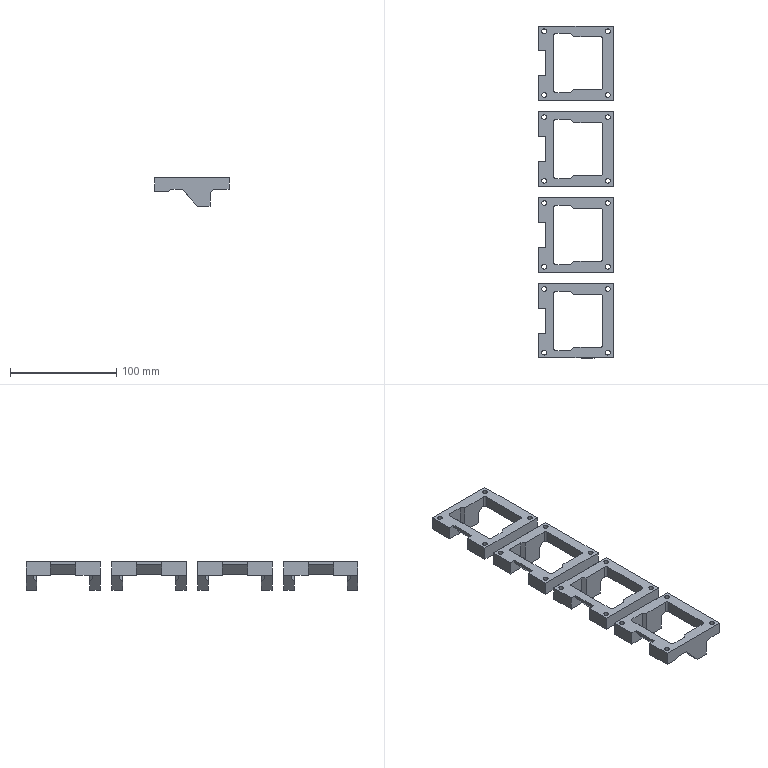NC program | NX | posted with a generic post | part box 70 x 313 x 26.9 mm
Lines 24 to 1089 of 34421:
(CAVITY_MILL , TOOL : D10)
N46 T10 M6
N48 G54
N50 G17 G0 G90 X44.83 Y-46.995 S9500 M3
N52 G43 Z30. H10
N54 Z0.603
N56 G94 G1 Z-0.397 F1000.
N58 X41.366 Y-40.995
N60 G3 X40.5 Y-40.495 R1.
N62 G1 X-171.505 F3000.
N64 G2 X-171.996 Y-40.004 R0.491
N66 G1 Y40.004
N68 G2 X-171.505 Y40.495 R0.491
N70 G1 X171.505
N72 G2 X171.996 Y40.004 R0.491
N74 G1 Y-40.004
N76 G2 X171.505 Y-40.495 R0.491
N78 G1 X40.5
N80 Y-33.495
N82 X-164.996
N84 Y33.495
N86 X164.996
N88 Y-33.495
N90 X40.5
N92 Y-26.495
N94 X-157.996
N96 Y-23.326
N98 G3 X-156.5 Y-23.5 R6.5
N100 G1 X-146.5
N102 G3 X-144.444 Y-23.166 R6.5
N104 X-143.618 Y-22.826 R6.5
N106 X-143.07 Y-22.521 R6.5
N108 X-141.163 Y-20.711 R6.5
N110 X-140. Y-17. R6.5
N112 G1 Y-4.563
N114 G3 X-146.5 Y1.969 R6.527
N116 G1 X-156.5
N118 G3 X-157.996 Y1.788 R6.53
N120 G1 X-157.669 Y0.427
N122 G2 X-156.5 Y0.569 R5.13
N124 G1 X-146.5
N126 G2 X-141.4 Y-4.563 R5.127
N128 G1 Y-17.
N130 G2 X-142.307 Y-19.903 R5.1
N132 G1 X-142.36 Y-19.979
N134 G2 X-143.797 Y-21.325 R5.1
N136 G1 X-143.905 Y-21.39
N138 G2 X-144.877 Y-21.835 R5.1
N140 G1 X-144.973 Y-21.866
N142 G2 X-146.5 Y-22.1 R5.1
N144 G1 X-156.5
N146 G2 X-161.6 Y-17. R5.1
N148 G1 Y-4.563
N150 G2 X-157.669 Y0.427 R5.13
N152 G1 X-157.996 Y1.788
N154 Y26.495
N156 X157.996
N158 Y1.788
N160 G3 X156.5 Y1.969 R6.53
N162 G1 X146.5
N164 G3 X140. Y-4.565 R6.527
N166 G1 Y-17.
N168 G3 X143.34 Y-22.68 R6.5
N170 X146.5 Y-23.5 R6.5
N172 G1 X156.5
N174 G3 X157.996 Y-23.326 R6.5
N176 G1 X157.674 Y-21.963
N178 G2 X156.5 Y-22.1 R5.1
N180 G1 X146.5
N182 G2 X144.02 Y-21.457 R5.1
N184 X141.4 Y-17. R5.1
N186 G1 Y-4.563
N188 G2 X146.5 Y0.569 R5.127
N190 G1 X156.5
N192 G2 X161.6 Y-4.563 R5.13
N194 G1 Y-17.179
N196 X161.593 Y-17.274
N198 G2 X157.674 Y-21.963 R5.1
N200 G1 X157.996 Y-23.326
N202 Y-26.495
N204 X40.5
N206 Y-19.495
N208 X21.501
N210 G3 X21.99 Y-17.356 R6.5
N212 X22. Y-17. R6.5
N214 G1 Y-4.566
N216 G3 X15.504 Y1.969 R6.516
N218 G1 X5.496
N220 G3 X0. Y-1.078 R6.516
N222 G1 X1.185 Y-1.824
N224 G2 X5.5 Y0.569 R5.116
N226 G1 X15.5
N228 G2 X20.6 Y-4.563 R5.116
N230 G1 Y-17.
N232 G2 X20.593 Y-17.261 R5.1
N234 G1 X20.567 Y-17.579
N236 G2 X18.573 Y-21.07 R5.1
N238 G1 X18.133 Y-21.368
N240 G2 X15.5 Y-22.1 R5.1
N242 G1 X5.5
N244 G2 X0.4 Y-17. R5.1
N246 G1 Y-4.563
N248 G2 X1.185 Y-1.824 R5.116
N250 G1 X0. Y-1.078
N252 G3 X-5.496 Y1.969 R6.516
N254 G1 X-15.504
N256 G3 X-22. Y-4.566 R6.516
N258 G1 Y-17.
N260 G3 X-21.502 Y-19.495 R6.5
N262 G1 X-20.209 Y-18.958
N264 G2 X-20.6 Y-17. R5.1
N266 G1 Y-4.563
N268 G2 X-15.5 Y0.569 R5.116
N270 G1 X-5.5
N272 G2 X-0.4 Y-4.563 R5.116
N274 G1 Y-17.
N276 G2 X-2.319 Y-20.987 R5.1
N278 G1 X-3.093 Y-21.495
N280 X-3.141 Y-21.521
N282 G2 X-5.5 Y-22.1 R5.1
N284 G1 X-15.5
N286 G2 X-17.831 Y-21.536 R5.1
N288 X-20.209 Y-18.958 R5.1
N290 G1 X-21.502 Y-19.495
N292 X-59.498
N294 G3 X-59.006 Y-17.316 R6.5
N296 G1 X-59. Y-17.19
N298 Y-4.563
N300 G3 X-65.5 Y1.969 R6.525
N302 G1 X-75.5
N304 G3 X-81. Y-1.078 R6.516
N306 G1 X-79.815 Y-1.824
N308 G2 X-75.5 Y0.569 R5.116
N310 G1 X-65.481
N312 G2 X-60.4 Y-4.563 R5.125
N314 G1 Y-17.19
N316 X-60.407 Y-17.269
N318 G2 X-60.816 Y-19.017 R5.1
N320 G1 X-60.881 Y-19.161
N322 G2 X-64.755 Y-22.045 R5.1
N324 G1 X-65.5 Y-22.1
N326 X-75.5
N328 G2 X-80.6 Y-17. R5.1
N330 G1 Y-4.563
N332 G2 X-79.815 Y-1.824 R5.116
N334 G1 X-81. Y-1.078
N336 G3 X-86.5 Y1.969 R6.516
N338 G1 X-96.504
N340 G3 X-103. Y-4.566 R6.516
N342 G1 Y-17.
N344 G3 X-102.502 Y-19.495 R6.5
N346 G1 X-101.209 Y-18.958
N348 G2 X-101.6 Y-17. R5.1
N350 G1 Y-4.563
N352 G2 X-96.5 Y0.569 R5.116
N354 G1 X-86.5
N356 G2 X-81.4 Y-4.563 R5.116
N358 G1 Y-17.
N360 G2 X-85.106 Y-21.906 R5.1
N362 G1 X-85.332 Y-21.964
N364 X-85.437 Y-21.988
N366 X-85.583 Y-22.017
N368 X-85.867 Y-22.061
N370 G2 X-86.5 Y-22.1 R5.1
N372 G1 X-96.5
N374 X-97.185 Y-22.054
N376 G2 X-97.573 Y-21.986 R5.1
N378 G1 X-97.719 Y-21.952
N380 X-97.816 Y-21.927
N382 G2 X-101.209 Y-18.958 R5.1
N384 G1 X-102.502 Y-19.495
N386 X-133.233
N388 G3 X-133. Y-17. R13.5
N390 G1 Y-4.566
N392 G3 X-146.486 Y8.969 R13.527
N394 G1 X-150.996
N396 Y19.495
N398 X150.996
N400 Y8.969
N402 X146.486
N404 G3 X133. Y-4.569 R13.527
N406 G1 Y-17.
N408 G3 X133.233 Y-19.495 R13.5
N410 G1 X102.501
N412 G3 X103. Y-17. R6.5
N414 G1 Y-4.566
N416 G3 X96.5 Y1.969 R6.516
N418 G1 X86.5
N420 G3 X81. Y-1.078 R6.516
N422 G1 X82.185 Y-1.824
N424 G2 X86.5 Y0.569 R5.116
N426 G1 X96.5
N428 G2 X101.6 Y-4.563 R5.116
N430 G1 Y-17.
N432 G2 X101.061 Y-19.282 R5.1
N434 G1 X100.899 Y-19.581
N436 G2 X96.5 Y-22.1 R5.1
N438 G1 X86.5
N440 G2 X81.4 Y-17. R5.1
N442 G1 Y-4.563
N444 G2 X82.185 Y-1.824 R5.116
N446 G1 X81. Y-1.078
N448 G3 X75.504 Y1.969 R6.516
N450 G1 X65.496
N452 G3 X59. Y-4.565 R6.516
N454 G1 Y-17.
N456 G3 X59.009 Y-17.339 R6.5
N458 X59.498 Y-19.495 R6.5
N460 G1 X60.791 Y-18.958
N462 G2 X60.408 Y-17.279 R5.1
N464 G1 X60.402 Y-17.159
N466 X60.4 Y-17.
N468 Y-4.563
N470 G2 X65.5 Y0.569 R5.116
N472 G1 X75.5
N474 G2 X80.6 Y-4.563 R5.116
N476 G1 Y-17.
N478 G2 X75.5 Y-22.1 R5.1
N480 G1 X65.5
N482 G2 X63.785 Y-21.803 R5.1
N484 X60.791 Y-18.958 R5.1
N486 G1 X59.498 Y-19.495
N488 X40.5
N490 Y-12.495
N492 X29.
N494 Y-4.574
N496 G3 X15.516 Y8.969 R13.516
N498 G1 X5.484
N500 G3 X0. Y7.792 R13.516
N502 X-5.484 Y8.969 R13.516
N504 G1 X-15.516
N506 G3 X-29. Y-4.574 R13.516
N508 G1 Y-12.495
N510 X-52.
N512 Y-4.567
N514 G3 X-65.487 Y8.969 R13.525
N516 G1 X-75.509
N518 G3 X-81. Y7.792 R13.516
N520 X-86.491 Y8.969 R13.516
N522 G1 X-96.516
N524 G3 X-110. Y-4.574 R13.516
N526 G1 Y-12.495
N528 X-126.
N530 Y-4.568
N532 G3 X-135.101 Y12.495 R20.527
N534 G1 X-142.337 Y13.968
N536 X-135.101 Y12.495
N538 X-114.374
N540 Y5.495
N542 G3 X-117. Y-4.58 R20.516
N544 G1 Y-5.495
N546 X-119.
N548 Y-4.57
N550 G3 X-120.901 Y5.495 R27.527
N552 G1 X-114.374
N554 Y12.495
N556 X-33.374
N558 Y5.495
N560 G3 X-36. Y-4.58 R20.516
N562 G1 Y-5.495
N564 X-45.
N566 Y-4.57
N568 G3 X-47.629 Y5.495 R20.525
N570 G1 X-33.374
N572 X-39.878 Y0.995
N574 G3 X-40.247 Y-0.995 R25.016
N576 G1 X-40.755
N578 G3 X-41.123 Y0.995 R25.025
N580 G1 X-39.878
N582 X-33.374 Y5.495
N584 Y12.495
N586 X135.101
N588 X142.337 Y13.968
N590 X135.101 Y12.495
N592 G3 X126. Y-4.571 R20.527
N594 G1 Y-12.495
N596 X110.
N598 Y-4.574
N600 G3 X108.27 Y2.069 R13.516
N602 G1 X114.374 Y5.495
N604 X120.901
N606 G3 X119. Y-4.574 R27.527
N608 G1 Y-5.495
N610 X117.
N612 Y-4.58
N614 G3 X114.374 Y5.495 R20.516
N616 G1 X108.27 Y2.069
N618 G3 X96.509 Y8.969 R13.516
N620 G1 X86.491
N622 G3 X81. Y7.792 R13.516
N624 X75.516 Y8.969 R13.516
N626 G1 X65.484
N628 G3 X52. Y-4.574 R13.516
N630 G1 Y-12.495
N632 X40.5
N634 Y-5.495
N636 X36.
N638 Y-4.58
N640 G3 X33.374 Y5.495 R20.516
N642 G1 X47.626
N644 G3 X45. Y-4.58 R20.516
N646 G1 Y-5.495
N648 X40.5
N650 Y-0.995
N652 X40.247
N654 G3 X39.878 Y0.995 R25.016
N656 G1 X41.122
N658 G3 X40.753 Y-0.995 R25.016
N660 G1 X40.5
N662 G3 X39.634 Y-1.495 R1.
N664 G1 Z0.603
N666 G0 Z30.
N668 X44.83 Y-46.995
N670 Z0.206
N672 G1 Z-0.794 F1000.
N674 X41.366 Y-40.995
N676 G3 X40.5 Y-40.495 R1.
N678 G1 X-171.505 F3000.
N680 G2 X-171.996 Y-40.004 R0.491
N682 G1 Y40.004
N684 G2 X-171.505 Y40.495 R0.491
N686 G1 X171.505
N688 G2 X171.996 Y40.004 R0.491
N690 G1 Y-40.004
N692 G2 X171.505 Y-40.495 R0.491
N694 G1 X40.5
N696 Y-33.495
N698 X-164.996
N700 Y33.495
N702 X164.996
N704 Y-33.495
N706 X40.5
N708 Y-26.495
N710 X-157.996
N712 Y-23.325
N714 G3 X-156.5 Y-23.5 R6.5
N716 G1 X-146.5
N718 G3 X-144.444 Y-23.166 R6.5
N720 X-143.618 Y-22.826 R6.5
N722 X-143.07 Y-22.521 R6.5
N724 X-141.217 Y-20.786 R6.5
N726 X-140. Y-17. R6.5
N728 G1 Y-4.22
N730 G3 X-146.5 Y2.314 R6.516
N732 G1 X-156.5
N734 G3 X-157.996 Y2.133 R6.533
N736 G1 X-157.668 Y0.772
N738 G2 X-156.5 Y0.914 R5.133
N740 G1 X-146.5
N742 G2 X-141.4 Y-4.218 R5.116
N744 G1 Y-17.
N746 G2 X-142.307 Y-19.903 R5.1
N748 G1 X-142.36 Y-19.979
N750 G2 X-143.797 Y-21.325 R5.1
N752 G1 X-143.905 Y-21.39
N754 G2 X-144.877 Y-21.835 R5.1
N756 G1 X-144.973 Y-21.866
N758 G2 X-146.5 Y-22.1 R5.1
N760 G1 X-156.5
N762 G2 X-161.6 Y-17. R5.1
N764 G1 Y-4.218
N766 G2 X-157.668 Y0.772 R5.133
N768 G1 X-157.996 Y2.133
N770 Y26.495
N772 X157.996
N774 Y2.133
N776 G3 X156.5 Y2.314 R6.533
N778 G1 X146.5
N780 G3 X140. Y-4.22 R6.516
N782 G1 Y-17.
N784 G3 X143.34 Y-22.68 R6.5
N786 X146.5 Y-23.5 R6.5
N788 G1 X156.5
N790 G3 X157.996 Y-23.325 R6.5
N792 G1 X157.674 Y-21.963
N794 G2 X156.5 Y-22.1 R5.1
N796 G1 X146.5
N798 G2 X144.02 Y-21.457 R5.1
N800 X141.4 Y-17. R5.1
N802 G1 Y-4.218
N804 G2 X146.5 Y0.914 R5.116
N806 G1 X156.5
N808 G2 X161.6 Y-4.218 R5.133
N810 G1 Y-17.179
N812 X161.593 Y-17.274
N814 G2 X157.674 Y-21.963 R5.1
N816 G1 X157.996 Y-23.325
N818 Y-26.495
N820 X40.5
N822 Y-19.495
N824 X21.501
N826 G3 X21.99 Y-17.356 R6.5
N828 X22. Y-17. R6.5
N830 G1 Y-4.22
N832 G3 X15.5 Y2.314 R6.516
N834 G1 X5.5
N836 G3 X0. Y-0.741 R6.527
N838 G1 X1.186 Y-1.485
N840 G2 X5.5 Y0.914 R5.127
N842 G1 X15.5
N844 G2 X20.6 Y-4.218 R5.116
N846 G1 Y-17.
N848 G2 X20.593 Y-17.261 R5.1
N850 G1 X20.567 Y-17.579
N852 G2 X18.573 Y-21.07 R5.1
N854 G1 X18.133 Y-21.368
N856 G2 X15.5 Y-22.1 R5.1
N858 G1 X5.5
N860 G2 X0.4 Y-17. R5.1
N862 G1 Y-4.218
N864 G2 X1.186 Y-1.485 R5.127
N866 G1 X0. Y-0.741
N868 G3 X-5.5 Y2.314 R6.527
N870 G1 X-15.5
N872 G3 X-22. Y-4.22 R6.516
N874 G1 Y-17.
N876 G3 X-21.502 Y-19.495 R6.5
N878 G1 X-20.209 Y-18.958
N880 G2 X-20.6 Y-17. R5.1
N882 G1 Y-4.218
N884 G2 X-15.5 Y0.914 R5.116
N886 G1 X-5.5
N888 G2 X-0.4 Y-4.218 R5.127
N890 G1 Y-17.
N892 G2 X-2.319 Y-20.987 R5.1
N894 G1 X-3.093 Y-21.495
N896 X-3.141 Y-21.521
N898 G2 X-5.5 Y-22.1 R5.1
N900 G1 X-15.5
N902 G2 X-17.827 Y-21.538 R5.1
N904 X-20.209 Y-18.958 R5.1
N906 G1 X-21.502 Y-19.495
N908 X-59.498
N910 G3 X-59.006 Y-17.316 R6.5
N912 G1 X-59. Y-17.19
N914 Y-4.22
N916 G3 X-65.5 Y2.314 R6.516
N918 G1 X-75.5
N920 G3 X-80.999 Y-0.734 R6.52
N922 G1 X-79.814 Y-1.48
N924 G2 X-75.5 Y0.914 R5.12
N926 G1 X-65.5
N928 G2 X-60.4 Y-4.218 R5.116
N930 G1 Y-17.19
N932 X-60.407 Y-17.269
N934 G2 X-60.816 Y-19.017 R5.1
N936 G1 X-60.881 Y-19.161
N938 G2 X-64.755 Y-22.045 R5.1
N940 G1 X-65.5 Y-22.1
N942 X-75.5
N944 G2 X-80.6 Y-17. R5.1
N946 G1 Y-4.218
N948 G2 X-79.814 Y-1.48 R5.12
N950 G1 X-80.999 Y-0.734
N952 G3 X-86.5 Y2.314 R6.516
N954 G1 X-96.5
N956 G3 X-103. Y-4.22 R6.516
N958 G1 Y-17.
N960 G3 X-102.502 Y-19.495 R6.5
N962 G1 X-101.209 Y-18.958
N964 G2 X-101.6 Y-17. R5.1
N966 G1 Y-4.218
N968 G2 X-96.5 Y0.914 R5.116
N970 G1 X-86.5
N972 G2 X-81.4 Y-4.218 R5.116
N974 G1 Y-17.
N976 G2 X-85.106 Y-21.906 R5.1
N978 G1 X-85.332 Y-21.964
N980 X-85.437 Y-21.988
N982 X-85.583 Y-22.017
N984 X-85.867 Y-22.061
N986 G2 X-86.5 Y-22.1 R5.1
N988 G1 X-96.5
N990 X-97.185 Y-22.054
N992 G2 X-97.573 Y-21.986 R5.1
N994 G1 X-97.719 Y-21.952
N996 X-97.816 Y-21.927
N998 G2 X-101.209 Y-18.958 R5.1
N1000 G1 X-102.502 Y-19.495
N1002 X-133.233
N1004 G3 X-133. Y-17. R13.5
N1006 G1 Y-4.228
N1008 G3 X-146.491 Y9.314 R13.516
N1010 G1 X-150.996
N1012 Y19.495
N1014 X150.996
N1016 Y9.314
N1018 X146.491
N1020 G3 X133. Y-4.228 R13.516
N1022 G1 Y-17.
N1024 G3 X133.233 Y-19.495 R13.5
N1026 G1 X102.501
N1028 G3 X103. Y-17. R6.5
N1030 G1 Y-4.22
N1032 G3 X96.5 Y2.314 R6.516
N1034 G1 X86.5
N1036 G3 X80.999 Y-0.734 R6.516
N1038 G1 X82.185 Y-1.479
N1040 G2 X86.5 Y0.914 R5.116
N1042 G1 X96.5
N1044 G2 X101.6 Y-4.218 R5.116
N1046 G1 Y-17.
N1048 G2 X101.061 Y-19.282 R5.1
N1050 G1 X100.899 Y-19.581
N1052 G2 X96.5 Y-22.1 R5.1
N1054 G1 X86.5
N1056 G2 X81.4 Y-17. R5.1
N1058 G1 Y-4.218
N1060 G2 X82.185 Y-1.479 R5.116
N1062 G1 X80.999 Y-0.734
N1064 G3 X75.5 Y2.314 R6.52
N1066 G1 X65.5
N1068 G3 X59. Y-4.22 R6.516
N1070 G1 Y-17.
N1072 G3 X59.009 Y-17.339 R6.5
N1074 X59.498 Y-19.495 R6.5
N1076 G1 X60.791 Y-18.958
N1078 G2 X60.408 Y-17.279 R5.1
N1080 G1 X60.402 Y-17.159
N1082 X60.4 Y-17.
N1084 Y-4.218
N1086 G2 X65.5 Y0.914 R5.116
N1088 G1 X75.5
N1090 G2 X80.6 Y-4.218 R5.12
N1092 G1 Y-17.
N1094 G2 X75.5 Y-22.1 R5.1
N1096 G1 X65.5
N1098 G2 X63.785 Y-21.803 R5.1
N1100 X60.791 Y-18.958 R5.1
N1102 G1 X59.498 Y-19.495
N1104 X40.5
N1106 Y-12.495
N1108 X29.
N1110 Y-4.228
N1112 G3 X15.509 Y9.314 R13.516
N1114 G1 X5.485
N1116 G3 X0. Y8.134 R13.527
N1118 X-5.485 Y9.314 R13.527
N1120 G1 X-15.509
N1122 G3 X-29. Y-4.228 R13.516
N1124 G1 Y-12.495
N1126 X-52.
N1128 Y-4.228
N1130 G3 X-65.491 Y9.314 R13.516
N1132 G1 X-75.511
N1134 G3 X-80.999 Y8.137 R13.52
N1136 X-86.491 Y9.314 R13.516
N1138 G1 X-96.509
N1140 G3 X-110. Y-4.228 R13.516
N1142 G1 Y-12.495
N1144 X-126.
N1146 Y-4.235
N1148 G3 X-134.595 Y12.495 R20.516
N1150 G1 X-141.583 Y14.047
N1152 X-134.595 Y12.495
N1154 X-114.564
N1156 Y5.495
N1158 G3 X-117. Y-4.235 R20.516
N1160 G1 Y-5.495
N1162 X-119.
N1164 Y-4.24
N1166 G3 X-120.765 Y5.495 R27.516
N1168 G1 X-114.564
N1170 Y12.495
N1172 X-33.564
N1174 Y5.495
N1176 G3 X-36. Y-4.235 R20.516
N1178 G1 Y-5.495
N1180 X-45.
N1182 Y-4.235
N1184 G3 X-47.436 Y5.495 R20.516
N1186 G1 X-33.564
N1188 X-39.954 Y0.995
N1190 G3 X-40.294 Y-0.995 R25.016
N1192 G1 X-40.706
N1194 G3 X-41.046 Y0.995 R25.016
N1196 G1 X-39.954
N1198 X-33.564 Y5.495
N1200 Y12.495
N1202 X134.595
N1204 X141.583 Y14.047
N1206 X134.595 Y12.495
N1208 G3 X126. Y-4.235 R20.516
N1210 G1 Y-12.495
N1212 X110.
N1214 Y-4.228
N1216 G3 X108.395 Y2.187 R13.516
N1218 G1 X114.564 Y5.495
N1220 X120.765
N1222 G3 X119. Y-4.24 R27.516
N1224 G1 Y-5.495
N1226 X117.
N1228 Y-4.235
N1230 G3 X114.564 Y5.495 R20.516
N1232 G1 X108.395 Y2.187
N1234 G3 X96.509 Y9.314 R13.516
N1236 G1 X86.491
N1238 G3 X80.999 Y8.137 R13.516
N1240 X75.511 Y9.314 R13.52
N1242 G1 X65.491
N1244 G3 X52. Y-4.228 R13.516
N1246 G1 Y-12.495
N1248 X40.5
N1250 Y-5.495
N1252 X36.
N1254 Y-4.235
N1256 G3 X33.564 Y5.495 R20.516
N1258 G1 X47.436
N1260 G3 X45. Y-4.235 R20.516
N1262 G1 Y-5.495
N1264 X40.5
N1266 Y-0.995
N1268 X40.294
N1270 G3 X39.954 Y0.995 R25.016
N1272 G1 X41.046
N1274 G3 X40.706 Y-0.995 R25.016
N1276 G1 X40.5
N1278 G3 X39.634 Y-1.495 R1.
N1280 G1 Z0.206
N1282 G0 X44.83 Y-46.995 Z-0.191
N1284 G1 Z-1.191 F1000.
N1286 X41.366 Y-40.995
N1288 G3 X40.5 Y-40.495 R1.
N1290 G1 X-171.505 F3000.
N1292 G2 X-171.996 Y-40.004 R0.491
N1294 G1 Y40.004
N1296 G2 X-171.505 Y40.495 R0.491
N1298 G1 X171.505
N1300 G2 X171.996 Y40.004 R0.491
N1302 G1 Y-40.004
N1304 G2 X171.505 Y-40.495 R0.491
N1306 G1 X40.5
N1308 Y-33.495
N1310 X-164.996
N1312 Y33.495
N1314 X164.996
N1316 Y-33.495
N1318 X40.5
N1320 Y-26.495
N1322 X-157.996
N1324 Y-23.325
N1326 G3 X-156.5 Y-23.5 R6.5
N1328 G1 X-146.5
N1330 G3 X-144.444 Y-23.166 R6.5
N1332 X-143.618 Y-22.826 R6.5
N1334 X-143.07 Y-22.521 R6.5
N1336 X-141.217 Y-20.786 R6.5
N1338 X-140. Y-17. R6.5
N1340 G1 Y-3.875
N1342 G3 X-146.5 Y2.66 R6.516
N1344 G1 X-156.5
N1346 G3 X-157.996 Y2.482 R6.516
N1348 G1 X-157.671 Y1.12
N1350 G2 X-156.5 Y1.26 R5.116
N1352 G1 X-146.5
N1354 G2 X-141.4 Y-3.873 R5.116
N1356 G1 Y-17.
N1358 G2 X-142.307 Y-19.903 R5.1
N1360 G1 X-142.36 Y-19.979
N1362 G2 X-143.797 Y-21.325 R5.1
N1364 G1 X-143.905 Y-21.39
N1366 G2 X-144.877 Y-21.835 R5.1
N1368 G1 X-144.973 Y-21.866
N1370 G2 X-146.5 Y-22.1 R5.1
N1372 G1 X-156.5
N1374 G2 X-161.6 Y-17. R5.1
N1376 G1 Y-3.873
N1378 G2 X-157.671 Y1.12 R5.116
N1380 G1 X-157.996 Y2.482
N1382 Y26.495
N1384 X157.996
N1386 Y2.482
N1388 G3 X156.5 Y2.66 R6.516
N1390 G1 X146.5
N1392 G3 X140. Y-3.875 R6.516
N1394 G1 Y-17.
N1396 G3 X143.34 Y-22.68 R6.5
N1398 X146.5 Y-23.5 R6.5
N1400 G1 X156.5
N1402 G3 X157.996 Y-23.325 R6.5
N1404 G1 X157.674 Y-21.963
N1406 G2 X156.5 Y-22.1 R5.1
N1408 G1 X146.5
N1410 G2 X144.02 Y-21.457 R5.1
N1412 X141.4 Y-17. R5.1
N1414 G1 Y-3.873
N1416 G2 X146.5 Y1.26 R5.116
N1418 G1 X156.5
N1420 G2 X161.6 Y-3.873 R5.116
N1422 G1 Y-17.179
N1424 X161.593 Y-17.274
N1426 G2 X157.674 Y-21.963 R5.1
N1428 G1 X157.996 Y-23.325
N1430 Y-26.495
N1432 X40.5
N1434 Y-19.495
N1436 X21.501
N1438 G3 X21.99 Y-17.356 R6.5
N1440 X22. Y-17. R6.5
N1442 G1 Y-3.875
N1444 G3 X15.5 Y2.66 R6.516
N1446 G1 X5.5
N1448 G3 X0. Y-0.397 R6.53
N1450 G1 X1.186 Y-1.142
N1452 G2 X5.5 Y1.26 R5.13
N1454 G1 X15.5
N1456 G2 X20.6 Y-3.873 R5.116
N1458 G1 Y-17.
N1460 G2 X20.593 Y-17.261 R5.1
N1462 G1 X20.567 Y-17.579
N1464 G2 X18.573 Y-21.07 R5.1
N1466 G1 X18.133 Y-21.368
N1468 G2 X15.5 Y-22.1 R5.1
N1470 G1 X5.5
N1472 G2 X0.4 Y-17. R5.1
N1474 G1 Y-3.873
N1476 G2 X1.186 Y-1.142 R5.13
N1478 G1 X0. Y-0.397
N1480 G3 X-5.5 Y2.66 R6.53
N1482 G1 X-15.5
N1484 G3 X-22. Y-3.873 R6.531
N1486 G1 Y-17.
N1488 G3 X-21.502 Y-19.495 R6.5
N1490 G1 X-20.209 Y-18.958
N1492 G2 X-20.6 Y-17. R5.1
N1494 G1 Y-3.873
N1496 G2 X-15.5 Y1.26 R5.131
N1498 G1 X-5.5
N1500 G2 X-0.4 Y-3.873 R5.13
N1502 G1 Y-17.
N1504 G2 X-2.246 Y-20.927 R5.1
N1506 G1 X-2.318 Y-20.986
N1508 G2 X-3.141 Y-21.521 R5.1
N1510 G1 X-3.239 Y-21.571
N1512 G2 X-5.5 Y-22.1 R5.1
N1514 G1 X-15.5
N1516 G2 X-17.822 Y-21.541 R5.1
N1518 X-20.209 Y-18.958 R5.1
N1520 G1 X-21.502 Y-19.495
N1522 X-59.498
N1524 G3 X-59.006 Y-17.316 R6.5
N1526 G1 X-59. Y-17.19
N1528 Y-3.875
N1530 G3 X-65.5 Y2.66 R6.516
N1532 G1 X-75.5
N1534 G3 X-81. Y-0.388 R6.516
N1536 G1 X-79.815 Y-1.133
N1538 G2 X-75.5 Y1.26 R5.116
N1540 G1 X-65.5
N1542 G2 X-60.4 Y-3.873 R5.116
N1544 G1 Y-17.19
N1546 X-60.407 Y-17.269
N1548 G2 X-60.816 Y-19.017 R5.1
N1550 G1 X-60.881 Y-19.161
N1552 G2 X-64.755 Y-22.045 R5.1
N1554 G1 X-65.5 Y-22.1
N1556 X-75.5
N1558 G2 X-80.6 Y-17. R5.1
N1560 G1 Y-3.873
N1562 G2 X-79.815 Y-1.133 R5.116
N1564 G1 X-81. Y-0.388
N1566 G3 X-86.5 Y2.66 R6.516
N1568 G1 X-96.5
N1570 G3 X-103. Y-3.875 R6.516
N1572 G1 Y-17.
N1574 G3 X-102.502 Y-19.495 R6.5
N1576 G1 X-101.209 Y-18.958
N1578 G2 X-101.6 Y-17. R5.1
N1580 G1 Y-3.873
N1582 G2 X-96.5 Y1.26 R5.116
N1584 G1 X-86.5
N1586 G2 X-81.4 Y-3.873 R5.116
N1588 G1 Y-17.
N1590 G2 X-85.106 Y-21.906 R5.1
N1592 G1 X-85.332 Y-21.964
N1594 X-85.437 Y-21.988
N1596 X-85.583 Y-22.017
N1598 X-85.867 Y-22.061
N1600 G2 X-86.5 Y-22.1 R5.1
N1602 G1 X-96.5
N1604 X-97.179 Y-22.055
N1606 G2 X-97.573 Y-21.986 R5.1
N1608 G1 X-97.719 Y-21.952
N1610 X-97.816 Y-21.927
N1612 G2 X-101.209 Y-18.958 R5.1
N1614 G1 X-102.502 Y-19.495
N1616 X-133.233
N1618 G3 X-133. Y-17. R13.5
N1620 G1 Y-3.883
N1622 G3 X-146.491 Y9.66 R13.516
N1624 G1 X-150.996
N1626 Y19.495
N1628 X150.996
N1630 Y9.66
N1632 X146.491
N1634 G3 X133. Y-3.883 R13.516
N1636 G1 Y-17.
N1638 G3 X133.233 Y-19.495 R13.5
N1640 G1 X102.501
N1642 G3 X103. Y-17. R6.5
N1644 G1 Y-3.875
N1646 G3 X96.5 Y2.66 R6.516
N1648 G1 X86.5
N1650 G3 X81. Y-0.388 R6.516
N1652 G1 X82.185 Y-1.133
N1654 G2 X86.5 Y1.26 R5.116
N1656 G1 X96.5
N1658 G2 X101.6 Y-3.873 R5.116
N1660 G1 Y-17.
N1662 G2 X101.061 Y-19.282 R5.1
N1664 G1 X100.899 Y-19.581
N1666 G2 X96.5 Y-22.1 R5.1
N1668 G1 X86.5
N1670 G2 X81.4 Y-17. R5.1
N1672 G1 Y-3.873
N1674 G2 X82.185 Y-1.133 R5.116
N1676 G1 X81. Y-0.388
N1678 G3 X75.5 Y2.66 R6.516
N1680 G1 X65.5
N1682 G3 X59. Y-3.875 R6.516
N1684 G1 Y-17.
N1686 G3 X59.009 Y-17.339 R6.5
N1688 X59.498 Y-19.495 R6.5
N1690 G1 X60.791 Y-18.958
N1692 G2 X60.408 Y-17.279 R5.1
N1694 G1 X60.402 Y-17.159
N1696 X60.4 Y-17.
N1698 Y-3.873
N1700 G2 X65.5 Y1.26 R5.116
N1702 G1 X75.5
N1704 G2 X80.6 Y-3.873 R5.116
N1706 G1 Y-17.
N1708 G2 X75.5 Y-22.1 R5.1
N1710 G1 X65.5
N1712 G2 X63.785 Y-21.803 R5.1
N1714 X60.791 Y-18.958 R5.1
N1716 G1 X59.498 Y-19.495
N1718 X40.5
N1720 Y-12.495
N1722 X29.
N1724 Y-3.883
N1726 G3 X15.509 Y9.66 R13.516
N1728 G1 X5.484
N1730 G3 X0. Y8.478 R13.53
N1732 X-5.484 Y9.66 R13.53
N1734 G1 X-15.517
N1736 G3 X-29. Y-3.875 R13.531
N1738 G1 Y-12.495
N1740 X-52.
N1742 Y-3.883
N1744 G3 X-65.491 Y9.66 R13.516
N1746 G1 X-75.509
N1748 G3 X-81. Y8.483 R13.516
N1750 X-86.491 Y9.66 R13.516
N1752 G1 X-96.509
N1754 G3 X-110. Y-3.883 R13.516
N1756 G1 Y-12.495
N1758 X-126.
N1760 Y-3.889
N1762 G3 X-134.125 Y12.495 R20.516
N1764 G1 X-140.454 Y14.068
N1766 X-134.125 Y12.495
N1768 X-114.745
N1770 Y5.495
N1772 G3 X-117. Y-3.89 R20.516
N1774 G1 Y-5.495
N1776 X-119.
N1778 Y-3.895
N1780 G3 X-120.638 Y5.495 R27.516
N1782 G1 X-114.745
N1784 Y12.495
N1786 X-33.739
N1788 Y5.495
N1790 G3 X-36. Y-3.876 R20.531
N1792 G1 Y-5.495
N1794 X-45.
N1796 Y-3.89
N1798 G3 X-47.255 Y5.495 R20.516
N1800 G1 X-33.739
N1802 X-40.022 Y0.995
N1804 G3 X-40.334 Y-0.995 R25.031
N1806 G1 X-40.664
N1808 G3 X-40.975 Y0.995 R25.016
N1810 G1 X-40.022
N1812 X-33.739 Y5.495
N1814 Y12.495
N1816 X134.125
N1818 X140.454 Y14.068
N1820 X134.125 Y12.495
N1822 G3 X126. Y-3.889 R20.516
N1824 G1 Y-12.495
N1826 X110.
N1828 Y-3.883
N1830 G3 X108.514 Y2.304 R13.516
N1832 G1 X114.745 Y5.495
N1834 X120.638
N1836 G3 X119. Y-3.895 R27.516
N1838 G1 Y-5.495
N1840 X117.
N1842 Y-3.889
N1844 G3 X114.745 Y5.495 R20.516
N1846 G1 X108.514 Y2.304
N1848 G3 X96.509 Y9.66 R13.516
N1850 G1 X86.491
N1852 G3 X81. Y8.483 R13.516
N1854 X75.509 Y9.66 R13.516
N1856 G1 X65.491
N1858 G3 X52. Y-3.883 R13.516
N1860 G1 Y-12.495
N1862 X40.5
N1864 Y-5.495
N1866 X36.
N1868 Y-3.889
N1870 G3 X33.745 Y5.495 R20.516
N1872 G1 X47.255
N1874 G3 X45. Y-3.889 R20.516
N1876 G1 Y-5.495
N1878 X40.5
N1880 Y-0.995
N1882 X40.336
N1884 G3 X40.025 Y0.995 R25.016
N1886 G1 X40.975
N1888 G3 X40.664 Y-0.995 R25.016
N1890 G1 X40.5
N1892 G3 X39.634 Y-1.495 R1.
N1894 G1 Z-0.191
N1896 G0 X44.83 Y-46.995 Z-0.589
N1898 G1 Z-1.589 F1000.
N1900 X41.366 Y-40.995
N1902 G3 X40.5 Y-40.495 R1.
N1904 G1 X-171.505 F3000.
N1906 G2 X-171.996 Y-40.004 R0.491
N1908 G1 Y40.004
N1910 G2 X-171.505 Y40.495 R0.491
N1912 G1 X171.505
N1914 G2 X171.996 Y40.004 R0.491
N1916 G1 Y-40.004
N1918 G2 X171.505 Y-40.495 R0.491
N1920 G1 X40.5
N1922 Y-33.495
N1924 X-164.996
N1926 Y33.495
N1928 X164.996
N1930 Y-33.495
N1932 X40.5
N1934 Y-26.495
N1936 X-157.996
N1938 Y-23.325
N1940 G3 X-156.5 Y-23.5 R6.5
N1942 G1 X-146.5
N1944 G3 X-144.444 Y-23.166 R6.5
N1946 X-143.618 Y-22.826 R6.5
N1948 X-143.07 Y-22.521 R6.5
N1950 X-141.217 Y-20.786 R6.5
N1952 X-140. Y-17. R6.5
N1954 G1 Y-3.53
N1956 G3 X-146.5 Y3.005 R6.516
N1958 G1 X-156.5
N1960 G3 X-157.996 Y2.824 R6.531
N1962 G1 X-157.669 Y1.463
N1964 G2 X-156.5 Y1.605 R5.131
N1966 G1 X-146.5
N1968 G2 X-141.4 Y-3.528 R5.116
N1970 G1 Y-17.
N1972 G2 X-142.307 Y-19.903 R5.1
N1974 G1 X-142.36 Y-19.979
N1976 G2 X-143.797 Y-21.325 R5.1
N1978 G1 X-143.905 Y-21.39
N1980 G2 X-144.877 Y-21.835 R5.1
N1982 G1 X-144.973 Y-21.866
N1984 G2 X-146.5 Y-22.1 R5.1
N1986 G1 X-156.5
N1988 G2 X-161.6 Y-17. R5.1
N1990 G1 Y-3.528
N1992 G2 X-157.669 Y1.463 R5.131
N1994 G1 X-157.996 Y2.824
N1996 Y26.495
N1998 X157.996
N2000 Y2.824
N2002 G3 X156.5 Y3.005 R6.532
N2004 G1 X146.5
N2006 G3 X140. Y-3.53 R6.516
N2008 G1 Y-17.
N2010 G3 X143.34 Y-22.68 R6.5
N2012 X146.5 Y-23.5 R6.5
N2014 G1 X156.5
N2016 G3 X157.996 Y-23.325 R6.5
N2018 G1 X157.674 Y-21.963
N2020 G2 X156.5 Y-22.1 R5.1
N2022 G1 X146.5
N2024 G2 X144.02 Y-21.457 R5.1
N2026 X141.4 Y-17. R5.1
N2028 G1 Y-3.528
N2030 G2 X146.5 Y1.605 R5.116
N2032 G1 X156.5
N2034 G2 X161.6 Y-3.528 R5.132
N2036 G1 Y-17.179
N2038 X161.593 Y-17.274
N2040 G2 X157.674 Y-21.963 R5.1
N2042 G1 X157.996 Y-23.325
N2044 Y-26.495
N2046 X40.5
N2048 Y-19.495
N2050 X21.501
N2052 G3 X21.99 Y-17.356 R6.5
N2054 X22. Y-17. R6.5
N2056 G1 Y-3.53
N2058 G3 X15.504 Y3.005 R6.516
N2060 G1 X5.493
N2062 G3 X0. Y-0.05 R6.527
N2064 G1 X1.185 Y-0.795
N2066 G2 X5.5 Y1.605 R5.127
N2068 G1 X15.512
N2070 G2 X20.6 Y-3.528 R5.116
N2072 G1 Y-17.
N2074 G2 X20.593 Y-17.261 R5.1
N2076 G1 X20.567 Y-17.579
N2078 G2 X18.573 Y-21.07 R5.1
N2080 G1 X18.133 Y-21.368
N2082 G2 X15.5 Y-22.1 R5.1
N2084 G1 X5.5
N2086 G2 X0.4 Y-17. R5.1
N2088 G1 Y-3.528
N2090 G2 X1.185 Y-0.795 R5.127
N2092 G1 X0. Y-0.05
N2094 G3 X-5.5 Y3.005 R6.527
N2096 G1 X-15.5
N2098 G3 X-22. Y-3.53 R6.516
N2100 G1 Y-17.
N2102 G3 X-21.502 Y-19.495 R6.5
N2104 G1 X-20.209 Y-18.958
N2106 G2 X-20.6 Y-17. R5.1
N2108 G1 Y-3.528
N2110 G2 X-15.5 Y1.605 R5.116
N2112 G1 X-5.5
N2114 G2 X-0.4 Y-3.528 R5.127
N2116 G1 Y-17.
N2118 G2 X-2.246 Y-20.927 R5.1
N2120 G1 X-2.318 Y-20.986
N2122 G2 X-3.141 Y-21.521 R5.1
N2124 G1 X-3.239 Y-21.571
N2126 G2 X-5.5 Y-22.1 R5.1
N2128 G1 X-15.5
N2130 G2 X-17.816 Y-21.544 R5.1
N2132 X-20.209 Y-18.958 R5.1
N2134 G1 X-21.502 Y-19.495
N2136 X-59.498
N2138 G3 X-59.006 Y-17.316 R6.5
N2140 G1 X-59. Y-17.19
N2142 Y-3.53
N2144 G3 X-65.5 Y3.005 R6.516
N2146 G1 X-75.5
N2148 G3 X-80.999 Y-0.044 R6.519
N2150 G1 X-79.814 Y-0.789
N2152 G2 X-75.5 Y1.605 R5.119
N2154 G1 X-65.5
N2156 G2 X-60.4 Y-3.528 R5.116
N2158 G1 Y-17.19
N2160 X-60.407 Y-17.269
N2162 G2 X-60.816 Y-19.017 R5.1
N2164 G1 X-60.881 Y-19.161
N2166 G2 X-64.755 Y-22.045 R5.1
N2168 G1 X-65.5 Y-22.1
N2170 X-75.5